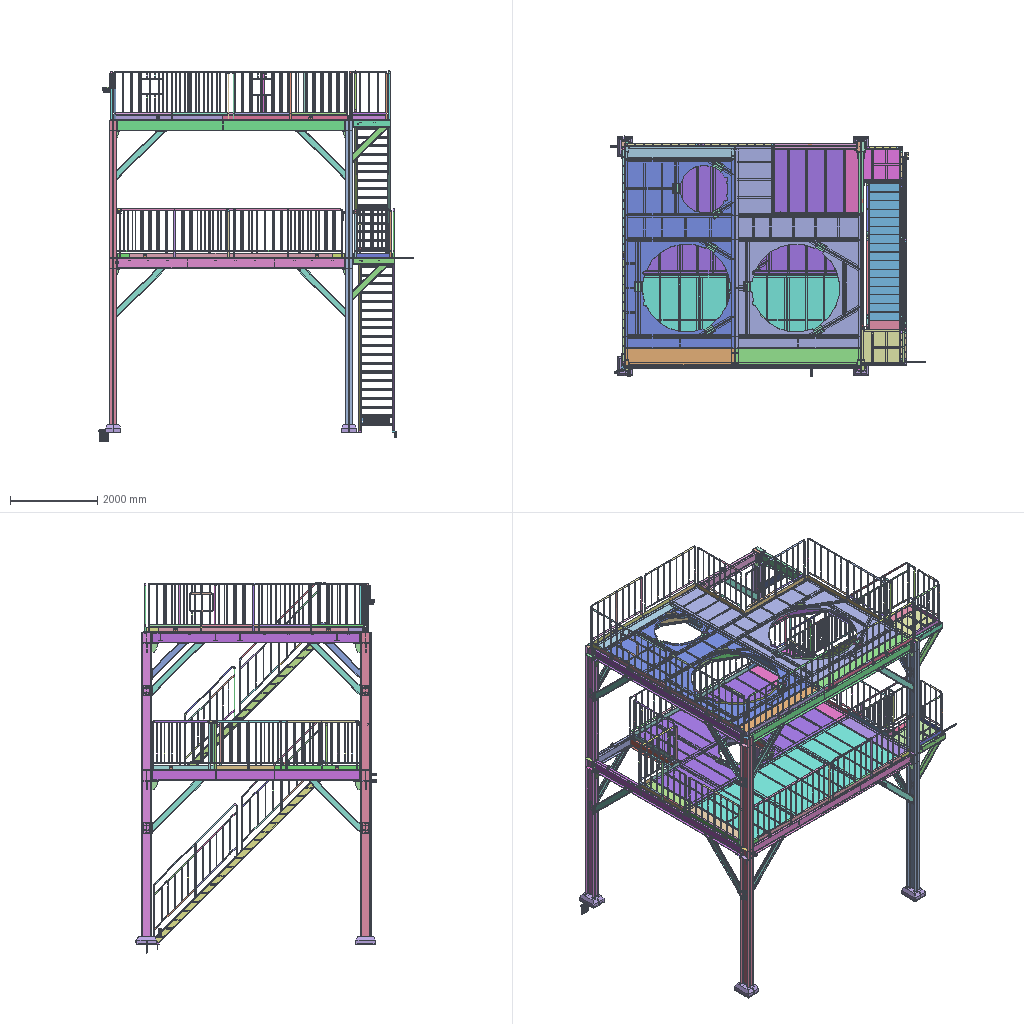Assembly | STEP file | 100 different items | 3011 placed | box 7212 x 5519 x 8479 mm
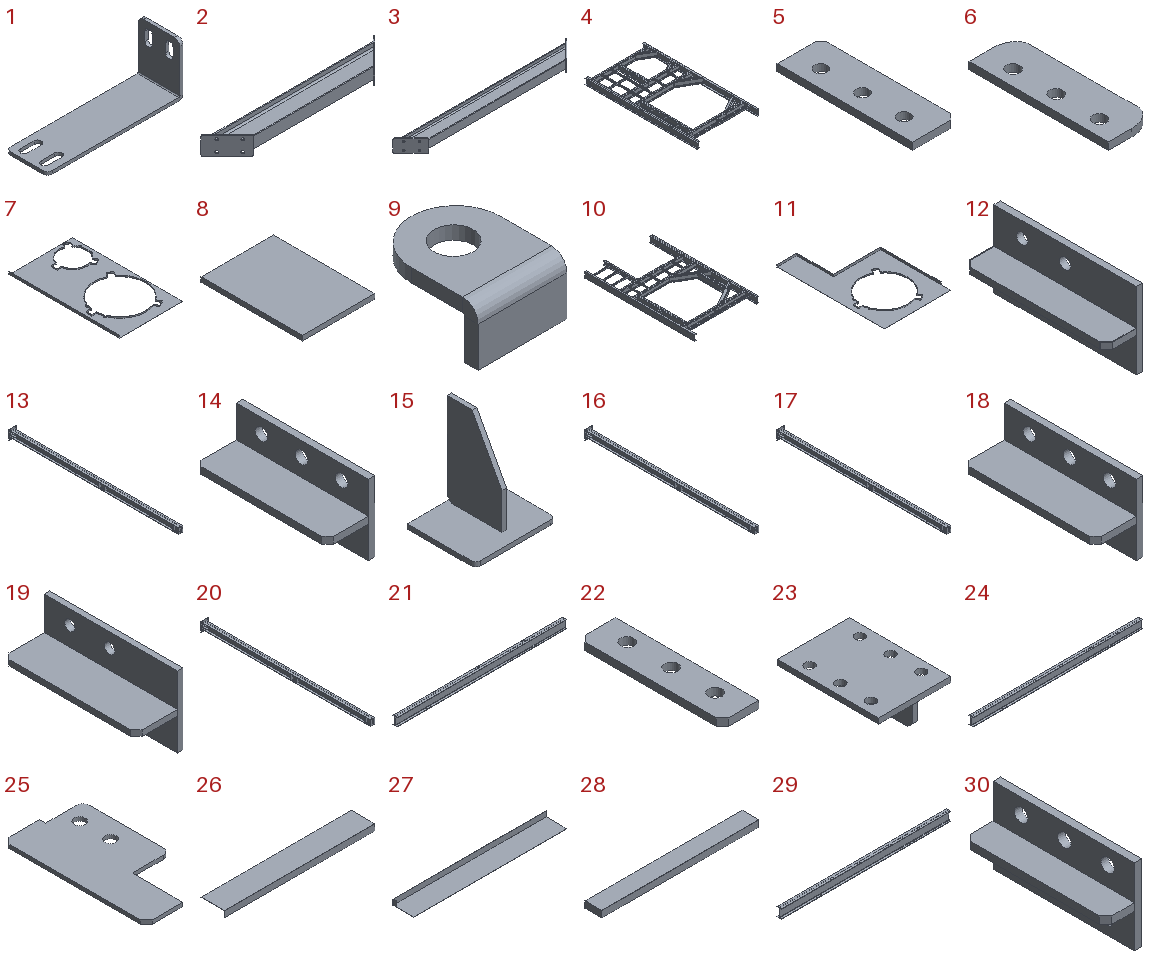Parts list (item | name | quantity | parent item | size | volume):
1 | PN_0061 L-type guardrail connecting plate 130X50_Default<As Machined> | x3 | - | 130 x 40 x 50 mm | 19703 mm3
2 | PN_0060 steel beam brace 1140_Default<As Machined> | x2 | - | 1178 x 182.434 x 125 mm | 2280023 mm3
3 | PN_0059 steel column and steel beam brace 1677_Default<As Machined> | x14 | - | 1715 x 182.434 x 125 mm | 3255129 mm3
4 | PN_0020 third-floor right platform 1_Default<As Machined> | x1 | in PN_0083 third-floor platform assembly 1 | 2578 x 4889 x 250 mm | 86538264 mm3
5 | PN_0021 flange connecting plate 12t_Default<As Machined> | x16 | in PN_0083 third-floor platform assembly 1, PN_0084 third-floor platform assembly 2, PN_0091 second-floor beam assembly, PN_0092 second-floor beam assembly 2 | 75 x 232 x 12 mm | 194530 mm3
6 | PN_0022 channel connecting plate 12t_Default<As Machined> | x8 | in PN_0083 third-floor platform assembly 1, PN_0084 third-floor platform assembly 2, PN_0093 second-floor platform assembly 1, PN_0094 second-floor platform assembly 2 | 73 x 226 x 12 mm | 180413 mm3
7 | PN_0023 third-floor right platform deck checkered steel plate_Default<As Machined> | x1 | in PN_0083 third-floor platform assembly 1 | 2515 x 4350 x 103 mm | 22833161 mm3
8 | PN_0009 support base plate 150x210_Default<As Machined> | x12 | in PN_0083 third-floor platform assembly 1, PN_0084 third-floor platform assembly 2, PN_0094 second-floor platform assembly 2 | 150 x 210 x 10 mm | 315000 mm3
9 | PN_0019 lifting lug _Default<As Machined> | x24 | in PN_0083 third-floor platform assembly 1, PN_0084 third-floor platform assembly 2, PN_0089 third-floor beam assembly 1, PN_0090 third-floor beam assembly 2, PN_0091 second-floor beam assembly, PN_0092 second-floor beam assembly 2, PN_0093 second-floor platform assembly 1, PN_0094 second-floor platform assembly 2 | 80 x 100 x 50 mm | 109398 mm3
10 | PN_0025 third-floor left platform 1_Default<As Machined> | x1 | in PN_0084 third-floor platform assembly 2 | 2948 x 4889 x 250 mm | 85593923 mm3
11 | PN_0024 third-floor left platform deck_Default<As Machined> | x1 | in PN_0084 third-floor platform assembly 2 | 2885 x 4620 x 103 mm | 23616795 mm3
12 | PN_0026 stair beam corbel 10t_Default<As Machined> | x3 | in PN_0084 third-floor platform assembly 2, PN_0092 second-floor beam assembly 2 | 59.5 x 233 x 125 mm | 507501 mm3
13 | PN_0027 steel column HM250X175=7134_Default<As Machined> | x1 | in PN_0085 column assembly 1 | 300 x 7150 x 400 mm | 42980324 mm3
14 | PN_0028 web-top 12t steel corbel_Default<As Machined> | x7 | in PN_0085 column assembly 1, PN_0086 column assembly 2, PN_0087 column assembly 3, PN_0088 column assembly 4 | 84 x 234 x 125 mm | 525836 mm3
15 | PN_0029 web-top 10t steel corbel_Default<As Machined> | x16 | in PN_0085 column assembly 1, PN_0086 column assembly 2, PN_0087 column assembly 3, PN_0088 column assembly 4 | 175 x 150 x 209.905 mm | 462571 mm3
16 | PN_0027 steel column HM250X175=7134_Default<As Machined> | x1 | in PN_0086 column assembly 2 | 300 x 7150 x 400 mm | 42979753 mm3
17 | PN_0027 steel column HM250X175=7134_Default<As Machined> | x1 | in PN_0087 column assembly 3 | 300 x 7150 x 400 mm | 42973088 mm3
18 | PN_0028 web-top 12t steel corbel_Default<As Machined> | x1 | in PN_0087 column assembly 3 | 84 x 234 x 125 mm | 525821 mm3
19 | PN_0030 stair beam corbel 10t_Default<As Machined> | x3 | in PN_0087 column assembly 3 | 82 x 234 x 125 mm | 449801 mm3
20 | PN_0027 steel column HM250X175=7134_Default<As Machined> | x1 | in PN_0088 column assembly 4 | 300 x 7150 x 400 mm | 42977522 mm3
21 | PN_0031 main beam HN250X125=5225_Default<As Machined> | x1 | in PN_0089 third-floor beam assembly 1 | 5225 x 125 x 250 mm | 19289440 mm3
22 | PN_0032 connecting plate 12t_Default<As Machined> | x20 | in PN_0089 third-floor beam assembly 1, PN_0090 third-floor beam assembly 2, PN_0093 second-floor platform assembly 1, PN_0094 second-floor platform assembly 2 | 59.5 x 232 x 12 mm | 151378 mm3
23 | PN_0033 beam connector 12t_Default<As Machined> | x4 | in PN_0089 third-floor beam assembly 1, PN_0090 third-floor beam assembly 2, PN_0091 second-floor beam assembly, PN_0092 second-floor beam assembly 2 | 164.5 x 232 x 59.5 mm | 562868 mm3
24 | PN_0031 main beam HN250X125=5225_Default<As Machined> | x1 | in PN_0090 third-floor beam assembly 2 | 5225 x 125 x 250 mm | 19288459 mm3
25 | PN_0034 channel connecting plate_Default<As Machined> | x1 | in PN_0090 third-floor beam assembly 2 | 119.5 x 232 x 6 mm | 129313 mm3
26 | PN_0035 third-floor site mounting plate 1_Default<As Machined> | x1 | - | 2515 x 394 x 103 mm | 3844530 mm3
27 | PN_0036 third-floor site mounting plate 2_Default<As Machined> | x1 | - | 2885 x 394 x 103 mm | 4292084 mm3
28 | PN_0037 third-floor site mounting plate 3_Default<As Machined> | x1 | - | 2515 x 270 x 103 mm | 2871750 mm3
29 | PN_0038 main beam HN250X125=5225_Default<As Machined> | x1 | in PN_0091 second-floor beam assembly | 4770 x 125 x 250 mm | 17605699 mm3
30 | PN_0039 web-top 12t steel corbel_Default<As Machined> | x2 | in PN_0091 second-floor beam assembly, PN_0092 second-floor beam assembly 2 | 59.5 x 232 x 125 mm | 452900 mm3
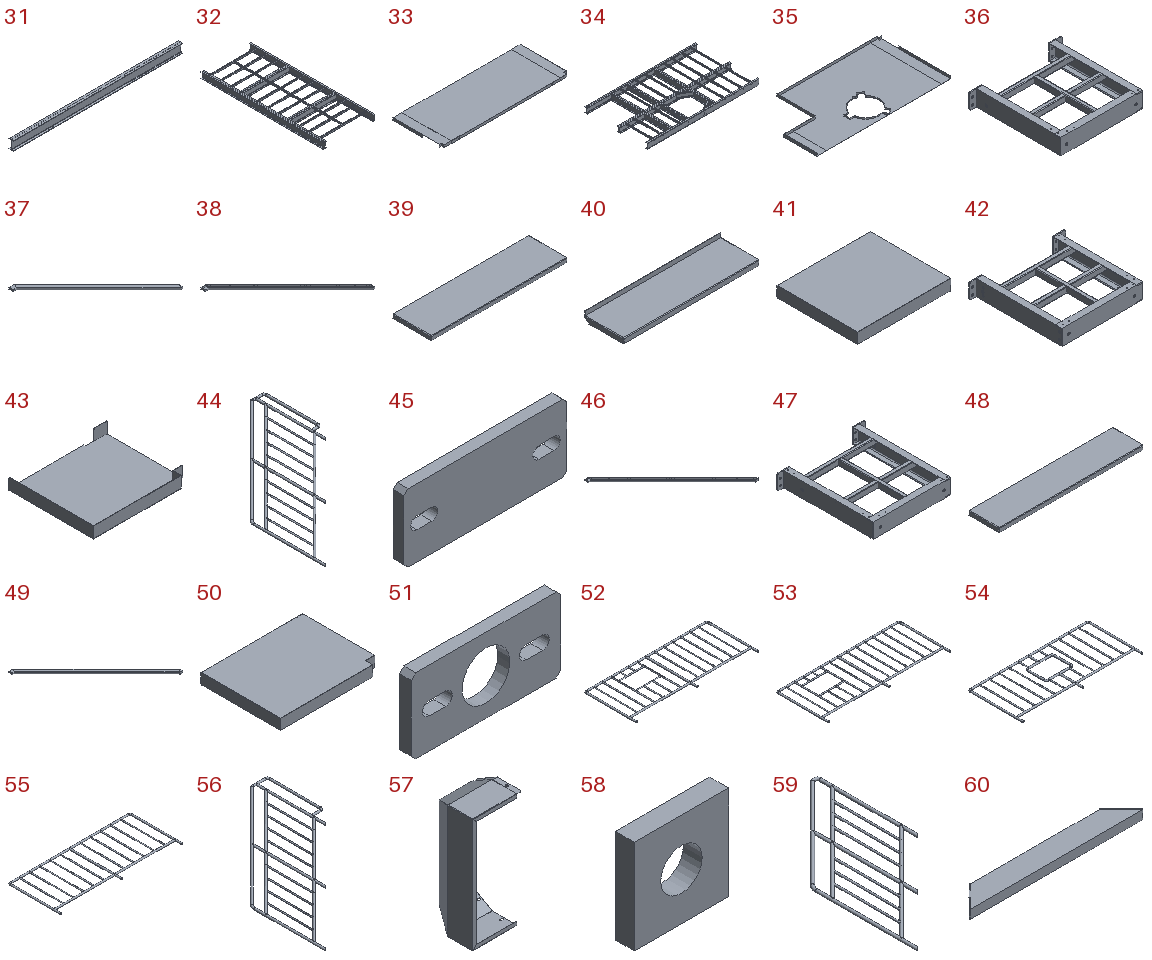31 | PN_0038 main beam HN250X125=5225_Default<As Machined> | x1 | in PN_0092 second-floor beam assembly 2 | 4770 x 125 x 250 mm | 17606026 mm3
32 | PN_0040 second-floor platform deck_Default<As Machined> | x1 | in PN_0093 second-floor platform assembly 1 | 2148 x 5275 x 250 mm | 68076276 mm3
33 | PN_0041 second-floor passage platform plate_Default<As Machined> | x1 | in PN_0093 second-floor platform assembly 1 | 5405 x 2088 x 103 mm | 36419067 mm3
34 | PN_0042 second-floor transition bin platform deck_Default<As Machined> | x1 | in PN_0094 second-floor platform assembly 2 | 5275 x 2990 x 250 mm | 103147929 mm3
35 | PN_0043 checkered steel plate 4785x1464_Default<As Machined> | x1 | in PN_0094 second-floor platform assembly 2 | 5405 x 2881 x 103 mm | 41382976 mm3
36 | PN_0044 steel stair platform_Default<As Machined> | x1 | in PN_0095 second-floor stair assembly | 951 x 886.002 x 160 mm | 6916698 mm3
37 | PN_0045 second-floor stair beam [16a_Default<As Machined> | x1 | in PN_0095 second-floor stair assembly | 3362 x 3310 x 63 mm | 10264966 mm3
38 | PN_0046 mirrored second-floor stair beam [16a_Default<As Machined> | x1 | in PN_0095 second-floor stair assembly | 3362 x 3310 x 63 mm | 10264966 mm3
39 | PN_0008 top 304 stair tread_Default<As Machined> | x1 | in PN_0095 second-floor stair assembly | 700 x 200 x 20 mm | 506035 mm3
40 | PN_0017 304 stair tread_Default<As Machined> | x35 | in PN_0095 second-floor stair assembly, PN_0098 first-floor steel stair assembly | 700 x 200 x 47 mm | 531503 mm3
41 | PN_0047 checkered steel plate 3_Default<As Machined> | x1 | in PN_0095 second-floor stair assembly | 891 x 771 x 103 mm | 2594390 mm3
42 | PN_0048 stair platform 2_Default<As Machined> | x1 | in PN_0096 stair platform assembly 2 | 951 x 886 x 160 mm | 6916619 mm3
43 | PN_0049 checkered steel plate 1_Default<As Machined> | x1 | in PN_0096 stair platform assembly 2 | 891 x 786 x 103 mm | 2627240 mm3
44 | PN_0050 stair guardrail B_Default<As Machined> | x2 | in PN_0097 first-floor stair guardrail A | 1972 x 2980 x 32 mm | 2990354 mm3
45 | PN_0013 304 stair handrail mounting plate 120X50X8_Default<As Machined> | x24 | in PN_0097 first-floor stair guardrail A, PN_0080 first-floor stair guardrail A, PN_0082 second-floor stair guardrail B, PN_0081 stair guardrail A section | 120 x 8 x 50 mm | 45254 mm3
46 | PN_0051 first-floor stair beam_Default<As Machined> | x1 | in PN_0098 first-floor steel stair assembly | 4058 x 4000 x 90 mm | 12422698 mm3
47 | PN_0052 steel stair platform 2_Default<As Machined> | x1 | in PN_0098 first-floor steel stair assembly | 951 x 986.002 x 160 mm | 7405397 mm3
48 | PN_0053 top 304 stair tread 2_Default<As Machined> | x1 | in PN_0098 first-floor steel stair assembly | 700 x 150 x 20 mm | 396167 mm3
49 | PN_0062 mirrored first-floor stair beam_Default<As Machined> | x1 | in PN_0098 first-floor steel stair assembly | 4058 x 4000 x 90 mm | 12422698 mm3
50 | PN_0054 checkered steel plate 2_Default<As Machined> | x1 | in PN_0098 first-floor steel stair assembly | 991 x 771 x 103 mm | 2887790 mm3
51 | PN_0067 304 guardrail mounting plate 100X50X8_Default<As Machined> | x67 | in PN_0099 304 guardrail 2600x1100B assembly, PN_0100 guardrail 2600x1100A assembly, PN_0101 304 guardrail 2400X1100A assembly, PN_0102 304 guardrail 2560X1100, PN_0065 304 guardrail 700X1100, PN_0079 platform deck guardrail 650x1100, PN_0076 304 guardrail 800X1100, PN_0064 304 guardrail 1950X1100, PN_0063 304 guardrail 1300X1100, PN_0070 304 guardrail 1150X1100, PN_0066 304 guardrail 1395X1100, PN_0068 304 guardrail 1880X1100, PN_0069 304 guardrail 1500X1100, PN_0078 304 guardrail 1620X1100, PN_0077 304 guardrail 2480X1100, PN_0075 304 guardrail 2400X1100 | 100 x 8 x 50 mm | 30820 mm3
52 | PN_0055 304 guardrail 2600X1100_Default<As Machined> | x1 | in PN_0099 304 guardrail 2600x1100B assembly | 2632 x 1116 x 32 mm | 2872572 mm3
53 | PN_0056 304 guardrail 2600X1100B_Default<As Machined> | x1 | in PN_0100 guardrail 2600x1100A assembly | 2632 x 1116 x 32 mm | 2870828 mm3
54 | PN_0057 304 guardrail 2400X1100 body A_Default<As Machined> | x1 | in PN_0101 304 guardrail 2400X1100A assembly | 2432 x 1116 x 32 mm | 2712212 mm3
55 | PN_0058 304 guardrail 2560X1100 body-A_Default<As Machined> | x1 | in PN_0102 304 guardrail 2560X1100 | 2592 x 1116 x 32 mm | 2611653 mm3
56 | PN_0012 stair guardrail B_Default<As Machined> | x2 | in PN_0080 first-floor stair guardrail A | 2022 x 2980 x 32 mm | 3009194 mm3
57 | PN_0018 H244x175 column protective cover_Default<As Machined> | x8 | - | 195 x 178.808 x 450 mm | 198447 mm3
58 | PN_0016 anchor bolt shim_Default<As Machined> | x40 | - | 50 x 10 x 50 mm | 21199 mm3
59 | PN_0015 second-floor stair guardrail A_Default<As Machined> | x2 | in PN_0082 second-floor stair guardrail B | 1170 x 2330 x 32 mm | 2093979 mm3
60 | PN_0010 stair platform brace 1257_Default<As Machined> | x3 | - | 1268 x 165.463 x 63 mm | 2607828 mm3
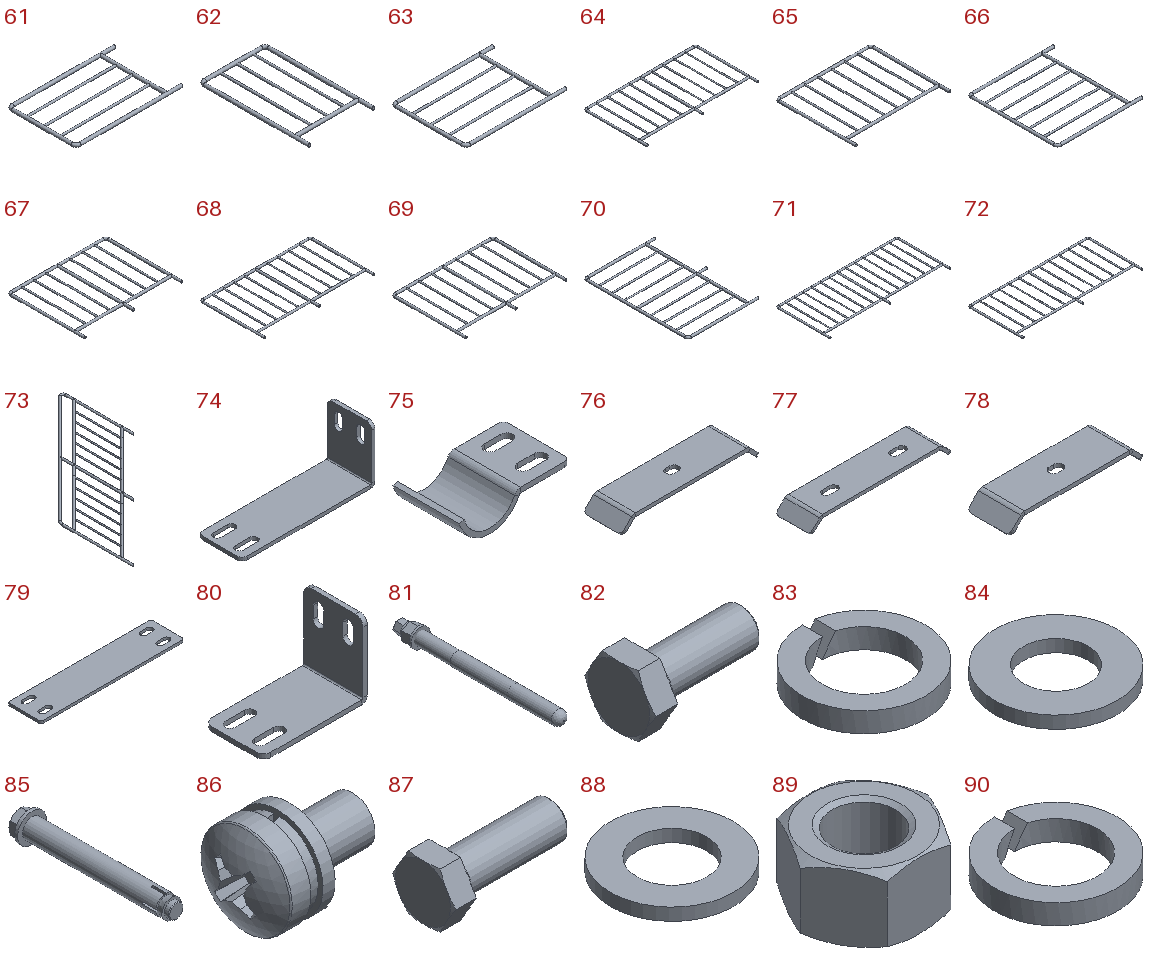61 | 304 guardrail 700X1100 body_Default<As Machined> | x1 | in PN_0065 304 guardrail 700X1100 | 1116 x 732 x 32 mm | 674327 mm3
62 | PN_0011 platform deck 304 guardrail 650X1100_Default<As Machined> | x3 | in PN_0079 platform deck guardrail 650x1100 | 682 x 1116 x 32 mm | 971799 mm3
63 | PN_0003 304 guardrail 800X1100 body-A_Default<As Machined> | x2 | in PN_0076 304 guardrail 800X1100 | 1116 x 832 x 32 mm | 1018076 mm3
64 | 304 guardrail 1950X1100-D body_Default<As Machined> | x2 | in PN_0064 304 guardrail 1950X1100 | 1982 x 1116 x 32 mm | 1461752 mm3
65 | 304 guardrail 1300X1100 body-B_Default<As Machined> | x1 | in PN_0063 304 guardrail 1300X1100 | 1332 x 1116 x 32 mm | 1011632 mm3
66 | 304 guardrail 1150X1100 body_Default<As Machined> | x1 | in PN_0070 304 guardrail 1150X1100 | 1116 x 1182 x 32 mm | 913541 mm3
67 | 304 guardrail 1395X1100 body B_Default<As Machined> | x1 | in PN_0066 304 guardrail 1395X1100 | 1427 x 1116 x 32 mm | 1755808 mm3
68 | 304 guardrail 1880X1100 body_Default<As Machined> | x1 | in PN_0068 304 guardrail 1880X1100 | 1912 x 1116 x 32 mm | 1441532 mm3
69 | 304 guardrail 1500X1100-B_Default<As Machined> | x2 | in PN_0069 304 guardrail 1500X1100 | 1532 x 1116 x 32 mm | 1222525 mm3
70 | PN_0005 guardrail 1620X1100 body_Default<As Machined> | x4 | in PN_0078 304 guardrail 1620X1100 | 1116 x 1652 x 32 mm | 1256893 mm3
71 | PN_0004 304 guardrail 2480X1100 body_Default<As Machined> | x2 | in PN_0077 304 guardrail 2480X1100 | 2512 x 1116 x 32 mm | 1834535 mm3
72 | PN_0002 304 guardrail 2400X1100 body-B_Default<As Machined> | x1 | in PN_0075 304 guardrail 2400X1100 | 2432 x 1116 x 32 mm | 2551384 mm3
73 | PN_0014 stair guardrail A_Default<As Machined> | x2 | in PN_0081 stair guardrail A section | 1927 x 3087 x 32 mm | 3023959 mm3
74 | PN_0007 L-type guardrail connecting plate 120X50_Default<As Machined> | x2 | - | 120 x 40 x 50 mm | 18503 mm3
75 | PN_0001 guardrail connecting plate 1_Default<As Machined> | x16 | in PN_0108 guardrail connection assembly 32 | 66.397 x 40 x 15 mm | 8448 mm3
76 | PN_0074 guardrail connecting plate (spacing 120)_Default<As Machined> | x120 | in PN_0110 guardrail connection assembly (spacing 120) 201 | 164.912 x 45 x 17 mm | 30539 mm3
77 | PN_0071 guardrail connecting plate (spacing 140)_Default<As Machined> | x12 | in PN_0107 guardrail connection assembly (spacing 140) 201 | 184.912 x 45 x 17 mm | 33225 mm3
78 | PN_0073 guardrail connecting plate (spacing 100)_Default<As Machined> | x16 | in PN_0109 guardrail connection assembly (spacing 100) 201 | 144.912 x 45 x 17 mm | 26939 mm3
79 | PN_0006 guardrail connecting plate 210_Default<As Machined> | x1 | - | 170 x 40 x 3 mm | 19243 mm3
80 | PN_0072 L-type guardrail connecting plate 70X50_Default<As Machined> | x1 | - | 70 x 40 x 50 mm | 12503 mm3
81 | Chemical anchor bolt M20X260 8.8 JBZQ4757-2006_Default<As Machined> | x40 | - | 30 x 262 x 30 mm | 79535 mm3
82 | Hex head bolt M8X20 A2-70 GBT5783-2016_GB_FASTENER_BOLT_STBAB A M8X20-N | x180 | in PN_0105 hex head bolt set M8X20 | 25.45 x 14.699 x 12.73 mm | 1753 mm3
83 | Spring washer 8 A2-70 GBT93-1987_GB_FASTENER_WASHER_SW 8 | x180 | in PN_0105 hex head bolt set M8X20 | 12.88 x 12.88 x 2.1 mm | 143.98 mm3
84 | Flat washer 8 A2-70 GBT97.1-2002_GB_FASTENER_WASHER_PWNA 8 | x240 | in PN_0105 hex head bolt set M8X20, PN_0106 hex head bolt set M8X50 | 16 x 16 x 1.6 mm | 233.031 mm3
85 | Cone-head expansion bolt (ZM type) M12×110 A2-70 GBT22795 (ZM) - 2008_Default<As Machined> | x6 | - | 24 x 129.18 x 24 mm | 26435 mm3
86 | Cross recessed pan head combination screw M6×12 A2-70 GBT9074.4-1988 | x20 | - | 16.483 x 12 x 12 mm | 913.256 mm3
87 | Hex head bolt M16X45 A2-70 GBT5783-2016_GB_FASTENER_BOLT_STBAB A M16X45-N | x200 | - | 55.18 x 27.332 x 23.67 mm | 13915 mm3
88 | Flat washer 16 A2-70 GBT97.1-2002_GB_FASTENER_WASHER_PWNA 16 | x200 | - | 30 x 30 x 3 mm | 1440 mm3
89 | Hex nut M16 A2-70 GBT6170-2015_GB_FASTENER_NUT_SNAB1 M16-N | x200 | - | 27.713 x 24 x 14.8 mm | 5071 mm3
90 | Spring washer 16 A2-70 GBT93-1987_GB_FASTENER_WASHER_SW 16 | x200 | - | 25.1 x 25.1 x 4.1 mm | 1069 mm3
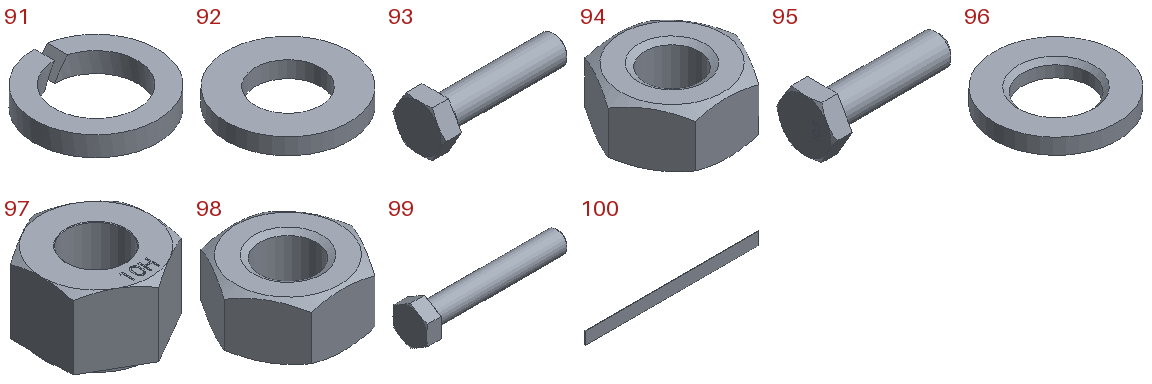91 | Spring washer 6 A2-70 GBT93-1987_GB_FASTENER_WASHER_SW 6 | x40 | in PN_0103 hex head bolt set M6X25 | 9.88 x 9.88 x 1.6 mm | 64.217 mm3
92 | Flat washer 6 A2-70 GBT97.1-2002_GB_FASTENER_WASHER_PWNA 6 | x40 | in PN_0103 hex head bolt set M6X25 | 12 x 12 x 1.6 mm | 129.484 mm3
93 | Hex head bolt M6X25 A2-70 GBT5783-2016_GB_FASTENER_BOLT_STBAB A M6X25-N | x40 | in PN_0103 hex head bolt set M6X25 | 29.15 x 11.293 x 9.78 mm | 1042 mm3
94 | Hex nut M6 A2-70 GBT6170-2015_GB_FASTENER_NUT_SNAB1 M6-N | x40 | in PN_0103 hex head bolt set M6X25 | 11.547 x 10 x 5.2 mm | 340.667 mm3
95 | Hex head bolt for steel structures M16×60 10.9 GBT1228-2006_M16×55 | x160 | in PN_0104 large hex head bolt set for steel structures M16X60 | 70.1 x 31.177 x 27 mm | 18177 mm3
96 | Washer for steel structures 16 GBT1230-2006_16 | x320 | in PN_0104 large hex head bolt set for steel structures M16X60 | 31.4 x 31.4 x 4 mm | 2155 mm3
97 | Hex nut for steel structures M16 10H GBT1229-2006_M16 | x160 | in PN_0104 large hex head bolt set for steel structures M16X60 | 25.6 x 29.56 x 17.2 mm | 7051 mm3
98 | Hex nut M8 A2-70 GBT6170-2015_GB_FASTENER_NUT_SNAB1 M8-N | x60 | in PN_0106 hex head bolt set M8X50 | 15.011 x 13 x 6.8 mm | 739.531 mm3
99 | Hex head bolt M8X50 A2-70 GBT5782-2016_GB_FASTENER_BOLT_SB A M8X40-C | x60 | in PN_0106 hex head bolt set M8X50 | 55.95 x 12.73 x 14.699 mm | 3330 mm3
100 | Stair anti-slip strip_Default<As Machined> | x80 | - | 700 x 3 x 50 mm | 105000 mm3
Placements (level | parent | child | x y z in mm | rotation matrix by rows), first 168 of 3581 lines:
1 | subassembly 2 | PN_0061 L-type guardrail connecting plate 130X50_Default<As Machined> | 4634.399 -2825.874 2881.2 | 1 0 0 0 0 -1 0 1 0
1 | subassembly 2 | PN_0061 L-type guardrail connecting plate 130X50_Default<As Machined> | 4634.399 2213.126 2881.2 | 1 0 0 0 0 -1 0 1 0
1 | subassembly 2 | PN_0061 L-type guardrail connecting plate 130X50_Default<As Machined> | -628.601 -2820.874 2881.2 | -1 0 0 0 0 -1 0 -1 -0
1 | subassembly 2 | PN_0060 steel beam brace 1140_Default<As Machined> | 4702.899 1802.641 4434.215 | 0 0 -1 0.7071 -0.7071 0 -0.7071 -0.7071 -0
1 | subassembly 2 | PN_0060 steel beam brace 1140_Default<As Machined> | 4702.899 -2357.389 4434.215 | 0 0 1 -0.7071 0.7071 0 -0.7071 -0.7071 -0
1 | subassembly 2 | PN_0059 steel column and steel beam brace 1677_Default<As Machined> | 4702.899 1612.783 1094.357 | 0 0 -1 0.7071 -0.7071 0 -0.7071 -0.7071 -0
1 | subassembly 2 | PN_0059 steel column and steel beam brace 1677_Default<As Machined> | 4702.899 -2167.531 1094.357 | 0 0 1 -0.7071 0.7071 0 -0.7071 -0.7071 0
1 | subassembly 2 | PN_0059 steel column and steel beam brace 1677_Default<As Machined> | 4204.556 -2784.374 1094.357 | 0.7071 -0.7071 0 0 0 1 -0.7071 -0.7071 -0
1 | subassembly 2 | PN_0059 steel column and steel beam brace 1677_Default<As Machined> | -697.101 -2167.531 1094.357 | 0 0 1 -0.7071 0.7071 0 -0.7071 -0.7071 -0
1 | subassembly 2 | PN_0059 steel column and steel beam brace 1677_Default<As Machined> | -198.758 2229.626 1094.357 | -0.7071 0.7071 0 0 0 -1 -0.7071 -0.7071 0
1 | subassembly 2 | PN_0059 steel column and steel beam brace 1677_Default<As Machined> | 4204.556 2229.626 1094.357 | 0.7071 -0.7071 0 0 0 1 -0.7071 -0.7071 -0
1 | subassembly 2 | PN_0059 steel column and steel beam brace 1677_Default<As Machined> | -198.758 -2784.374 1094.357 | -0.7071 0.7071 0 0 0 -1 -0.7071 -0.7071 0
1 | subassembly 2 | PN_0059 steel column and steel beam brace 1677_Default<As Machined> | -697.101 1612.783 1094.357 | 0 0 -1 0.7071 -0.7071 0 -0.7071 -0.7071 -0
1 | subassembly 2 | PN_0083 third-floor platform assembly 1 | 1225.628 -145.413 44.2 | 1 0 0 0 1 0 0 0 1
2 | PN_0083 third-floor platform assembly 1 | PN_0020 third-floor right platform 1_Default<As Machined> | -517.729 -869.961 4695.0 | 1 0 0 0 1 0 0 0 1
2 | PN_0083 third-floor platform assembly 1 | PN_0021 flange connecting plate 12t_Default<As Machined> | -1963.229 -2504.961 4820.0 | 1 0 0 0 0 -1 0 1 -0
2 | PN_0083 third-floor platform assembly 1 | PN_0021 flange connecting plate 12t_Default<As Machined> | -1882.229 -2516.961 4820.0 | -1 0 0 0 0 1 0 1 0
2 | PN_0083 third-floor platform assembly 1 | PN_0021 flange connecting plate 12t_Default<As Machined> | -1882.229 2253.039 4820.0 | -1 0 0 0 0 -1 0 -1 -0
2 | PN_0083 third-floor platform assembly 1 | PN_0021 flange connecting plate 12t_Default<As Machined> | -1963.229 2241.039 4820.0 | 1 0 0 0 0 1 0 -1 -0
2 | PN_0083 third-floor platform assembly 1 | PN_0022 channel connecting plate 12t_Default<As Machined> | 546.771 -2564.461 4820.0 | 1 0 0 0 0 -1 0 1 -0
2 | PN_0083 third-floor platform assembly 1 | PN_0022 channel connecting plate 12t_Default<As Machined> | 546.771 2312.539 4820.0 | 1 0 0 0 0 -1 0 1 -0
2 | PN_0083 third-floor platform assembly 1 | PN_0023 third-floor right platform deck checkered steel plate_Default<As Machined> | -517.729 -869.961 4948.0 | 1 0 0 0 1 0 0 0 1
2 | PN_0083 third-floor platform assembly 1 | PN_0009 support base plate 150x210_Default<As Machined> | 7.54 -1839.754 4955.0 | 0.5 -0.866 0 -0.866 -0.5 0 0 0 -1
2 | PN_0083 third-floor platform assembly 1 | PN_0009 support base plate 150x210_Default<As Machined> | -741.614 1419.392 4955.0 | 1 0 0 0 -1 0 0 0 -1
2 | PN_0083 third-floor platform assembly 1 | PN_0009 support base plate 150x210_Default<As Machined> | 59.502 69.832 4955.0 | 0.5 0.866 0 0.866 -0.5 0 0 0 -1
2 | PN_0083 third-floor platform assembly 1 | PN_0009 support base plate 150x210_Default<As Machined> | -1620.229 -839.961 4955.0 | -1 0 0 0 1 0 0 0 -1
2 | PN_0083 third-floor platform assembly 1 | PN_0009 support base plate 150x210_Default<As Machined> | 173.124 842.562 4955.0 | -0.5 0.866 0 0.866 0.5 0 0 0 -1
2 | PN_0083 third-floor platform assembly 1 | PN_0009 support base plate 150x210_Default<As Machined> | 215.304 1923.164 4955.0 | -0.5 -0.866 0 -0.866 0.5 0 0 0 -1
2 | PN_0083 third-floor platform assembly 1 | PN_0019 lifting lug _Default<As Machined> | -1947.729 1713.039 4957.0 | 0 0 1 1 0 0 0 1 0
2 | PN_0083 third-floor platform assembly 1 | PN_0019 lifting lug _Default<As Machined> | 571.271 2167.539 4880.118 | 0 -1 0 0 0 -1 1 0 0
2 | PN_0083 third-floor platform assembly 1 | PN_0019 lifting lug _Default<As Machined> | -1947.729 -1786.961 4957.0 | 0 0 1 1 0 0 0 1 0
2 | PN_0083 third-floor platform assembly 1 | PN_0019 lifting lug _Default<As Machined> | 571.271 -2332.461 4880.118 | 0 -1 0 0 0 -1 1 0 0
1 | subassembly 2 | PN_0084 third-floor platform assembly 2 | 3923.757 -499.454 44.2 | 1 0 0 0 1 0 0 0 1
2 | PN_0084 third-floor platform assembly 2 | PN_0025 third-floor left platform 1_Default<As Machined> | -715.858 -515.92 4695.0 | 1 0 0 0 1 0 0 0 1
2 | PN_0084 third-floor platform assembly 2 | PN_0021 flange connecting plate 12t_Default<As Machined> | 738.642 -2150.92 4820.0 | 1 0 0 0 0 -1 0 1 0
2 | PN_0084 third-floor platform assembly 2 | PN_0021 flange connecting plate 12t_Default<As Machined> | 819.642 -2150.92 4820.0 | -1 0 0 0 0 -1 0 -1 0
2 | PN_0084 third-floor platform assembly 2 | PN_0021 flange connecting plate 12t_Default<As Machined> | 819.642 2595.08 4820.0 | -1 0 0 0 0 1 0 1 0
2 | PN_0084 third-floor platform assembly 2 | PN_0021 flange connecting plate 12t_Default<As Machined> | 738.642 2607.08 4820.0 | 1 0 0 0 0 -1 0 1 -0
2 | PN_0084 third-floor platform assembly 2 | PN_0022 channel connecting plate 12t_Default<As Machined> | -2060.358 2654.58 4820.0 | -1 0 0 0 0 1 0 1 -0
2 | PN_0084 third-floor platform assembly 2 | PN_0022 channel connecting plate 12t_Default<As Machined> | -2060.358 -2222.42 4820.0 | -1 0 0 0 0 1 0 1 -0
2 | PN_0084 third-floor platform assembly 2 | PN_0024 third-floor left platform deck_Default<As Machined> | -715.858 -515.92 4948.0 | 1 0 0 0 1 0 0 0 1
2 | PN_0084 third-floor platform assembly 2 | PN_0009 support base plate 150x210_Default<As Machined> | -190.589 -1485.713 4945.0 | 0.5 0.866 0 -0.866 0.5 0 0 0 1
2 | PN_0084 third-floor platform assembly 2 | PN_0009 support base plate 150x210_Default<As Machined> | -138.627 423.873 4945.0 | 0.5 -0.866 0 0.866 0.5 0 0 0 1
2 | PN_0084 third-floor platform assembly 2 | PN_0009 support base plate 150x210_Default<As Machined> | -1818.358 -485.92 4945.0 | -1 0 0 0 -1 0 0 0 1
2 | PN_0084 third-floor platform assembly 2 | PN_0019 lifting lug _Default<As Machined> | 804.142 -1222.92 4957.0 | 0 0 -1 -1 0 0 0 1 0
2 | PN_0084 third-floor platform assembly 2 | PN_0019 lifting lug _Default<As Machined> | -2084.858 -2027.42 4880.118 | 0 1 0 0 0 1 1 0 -0
2 | PN_0084 third-floor platform assembly 2 | PN_0019 lifting lug _Default<As Machined> | -1080.858 1158.83 4884.0 | 0 0 1 0 1 0 -1 0 0
2 | PN_0084 third-floor platform assembly 2 | PN_0019 lifting lug _Default<As Machined> | 804.142 1477.08 4957.0 | 0 0 -1 -1 0 0 0 1 0
2 | PN_0084 third-floor platform assembly 2 | PN_0026 stair beam corbel 10t_Default<As Machined> | 806.892 -1452.971 4819 | 1 0 0 0 0 -1 0 1 0
1 | subassembly 2 | PN_0085 column assembly 1 | -697.101 2229.626 4989.2 | 1 0 0 0 0 1 0 -1 -0
2 | PN_0085 column assembly 1 | PN_0027 steel column HM250X175=7134_Default<As Machined> | -0.0 -0.0 -0.0 | 1 0 0 0 1 0 0 0 1
2 | PN_0085 column assembly 1 | PN_0028 web-top 12t steel corbel_Default<As Machined> | 39.5 125 6.004 | 1 0 0 0 -1 0 0 0 -1
2 | PN_0085 column assembly 1 | PN_0029 web-top 10t steel corbel_Default<As Machined> | 78.5 250.0 0.0 | 0 -1 0 0 0 1 -1 0 0
2 | PN_0085 column assembly 1 | PN_0028 web-top 12t steel corbel_Default<As Machined> | 39.5 3275 6.004 | 1 0 0 0 -1 0 0 0 -1
2 | PN_0085 column assembly 1 | PN_0029 web-top 10t steel corbel_Default<As Machined> | 78.5 3400.0 0.0 | 0 -1 0 0 0 1 -1 0 0
2 | PN_0085 column assembly 1 | PN_0029 web-top 10t steel corbel_Default<As Machined> | -0.0 250.0 -197.0 | -1 0 0 0 0 1 0 1 0
2 | PN_0085 column assembly 1 | PN_0029 web-top 10t steel corbel_Default<As Machined> | -0.0 3400.0 -197.0 | -1 0 0 0 0 1 0 1 0
1 | subassembly 2 | PN_0086 column assembly 2 | -950.144 4365.626 1027.473 | -1 0 0 0 0 -1 0 -1 0
2 | PN_0086 column assembly 2 | PN_0027 steel column HM250X175=7134_Default<As Machined> | -253.044 -3961.727 7150.0 | 1 0 0 0 1 0 0 0 1
2 | PN_0086 column assembly 2 | PN_0028 web-top 12t steel corbel_Default<As Machined> | -292.544 -3836.727 7143.996 | -1 0 0 0 -1 0 0 0 1
2 | PN_0086 column assembly 2 | PN_0029 web-top 10t steel corbel_Default<As Machined> | -331.541 -3711.727 7150.0 | 0 1 0 0 0 1 1 0 -0
2 | PN_0086 column assembly 2 | PN_0028 web-top 12t steel corbel_Default<As Machined> | -292.544 -686.727 7143.996 | -1 0 0 0 -1 0 0 0 1
2 | PN_0086 column assembly 2 | PN_0029 web-top 10t steel corbel_Default<As Machined> | -331.541 -561.727 7150.0 | 0 1 0 0 0 1 1 0 -0
2 | PN_0086 column assembly 2 | PN_0029 web-top 10t steel corbel_Default<As Machined> | -253.044 -3711.727 6953.0 | -1 0 0 0 0 1 0 1 0
2 | PN_0086 column assembly 2 | PN_0029 web-top 10t steel corbel_Default<As Machined> | -253.044 -561.727 6953.0 | -1 0 0 0 0 1 0 1 0
1 | subassembly 2 | PN_0087 column assembly 3 | 4449.855 4365.626 1027.473 | -1 0 0 0 0 -1 0 -1 -0
2 | PN_0087 column assembly 3 | PN_0027 steel column HM250X175=7134_Default<As Machined> | -253.044 -3961.727 7150.0 | 1 0 0 0 1 0 0 0 1
2 | PN_0087 column assembly 3 | PN_0028 web-top 12t steel corbel_Default<As Machined> | -213.544 -3836.727 7156.004 | 1 0 0 0 -1 0 0 0 -1
2 | PN_0087 column assembly 3 | PN_0029 web-top 10t steel corbel_Default<As Machined> | -174.544 -3711.727 7150.0 | 0 -1 0 0 0 1 -1 0 0
2 | PN_0087 column assembly 3 | PN_0028 web-top 12t steel corbel_Default<As Machined> | -213.544 -686.727 7156.004 | 1 0 0 0 -1 0 0 0 -1
2 | PN_0087 column assembly 3 | PN_0029 web-top 10t steel corbel_Default<As Machined> | -174.544 -561.727 7150.0 | 0 -1 0 0 0 1 -1 0 0
2 | PN_0087 column assembly 3 | PN_0029 web-top 10t steel corbel_Default<As Machined> | -253.044 -3711.727 6953.0 | -1 0 0 0 0 1 0 1 0
2 | PN_0087 column assembly 3 | PN_0029 web-top 10t steel corbel_Default<As Machined> | -253.044 -561.727 6953.0 | -1 0 0 0 0 1 0 1 0
2 | PN_0087 column assembly 3 | PN_0030 stair beam corbel 10t_Default<As Machined> | -294.544 -3836.727 7143.996 | -1 0 0 0 -1 0 0 0 1
2 | PN_0087 column assembly 3 | PN_0030 stair beam corbel 10t_Default<As Machined> | -294.544 -686.727 7143.996 | -1 0 0 0 -1 0 0 0 1
1 | subassembly 2 | PN_0088 column assembly 4 | 4955.943 -4920.374 1027.473 | 1 0 0 0 0 1 0 -1 -0
2 | PN_0088 column assembly 4 | PN_0027 steel column HM250X175=7134_Default<As Machined> | -253.044 -3961.727 7150.0 | 1 0 0 0 1 0 0 0 1
2 | PN_0088 column assembly 4 | PN_0028 web-top 12t steel corbel_Default<As Machined> | -292.544 -3836.727 7143.996 | -1 0 0 0 -1 0 0 0 1
2 | PN_0088 column assembly 4 | PN_0029 web-top 10t steel corbel_Default<As Machined> | -331.541 -3711.727 7150.0 | 0 1 0 0 0 1 1 0 -0
2 | PN_0088 column assembly 4 | PN_0028 web-top 12t steel corbel_Default<As Machined> | -292.544 -686.727 7143.996 | -1 0 0 0 -1 0 0 0 1
2 | PN_0088 column assembly 4 | PN_0029 web-top 10t steel corbel_Default<As Machined> | -331.541 -561.727 7150.0 | 0 1 0 0 0 1 1 0 -0
2 | PN_0088 column assembly 4 | PN_0029 web-top 10t steel corbel_Default<As Machined> | -253.044 -3711.727 6953.0 | -1 0 0 0 0 1 0 1 0
2 | PN_0088 column assembly 4 | PN_0029 web-top 10t steel corbel_Default<As Machined> | -253.044 -561.727 6953.0 | -1 0 0 0 0 1 0 1 0
1 | subassembly 2 | PN_0089 third-floor beam assembly 1 | 1784.52 -2781.678 -360.8 | -1 0 0 0 -1 0 0 0 1
2 | PN_0089 third-floor beam assembly 1 | PN_0031 main beam HN250X125=5225_Default<As Machined> | -2830.879 2.696 5225.0 | 1 0 0 0 1 0 0 0 1
2 | PN_0089 third-floor beam assembly 1 | PN_0032 connecting plate 12t_Default<As Machined> | -2830.879 35.446 5225.0 | 0 0 1 1 0 0 0 1 -0
2 | PN_0089 third-floor beam assembly 1 | PN_0032 connecting plate 12t_Default<As Machined> | 2382.121 35.446 5225.0 | 0 0 1 1 0 0 0 1 0
2 | PN_0089 third-floor beam assembly 1 | PN_0032 connecting plate 12t_Default<As Machined> | 2394.121 -30.054 5225.0 | 0 0 -1 -1 0 0 0 1 0
2 | PN_0089 third-floor beam assembly 1 | PN_0032 connecting plate 12t_Default<As Machined> | -2818.879 -30.054 5225.0 | 0 0 -1 -1 0 0 0 1 0
2 | PN_0089 third-floor beam assembly 1 | PN_0033 beam connector 12t_Default<As Machined> | -33.629 -47.804 5225.0 | 1 0 0 0 0 -1 0 1 -0
2 | PN_0089 third-floor beam assembly 1 | PN_0019 lifting lug _Default<As Machined> | -2040.879 30.196 5362.0 | 1 0 0 0 0 -1 0 1 -0
2 | PN_0089 third-floor beam assembly 1 | PN_0019 lifting lug _Default<As Machined> | 1459.121 30.196 5362.0 | 1 0 0 0 0 -1 0 1 -0
1 | subassembly 2 | PN_0090 third-floor beam assembly 2 | 1784.52 2232.322 -360.8 | -1 0 0 0 -1 0 0 0 1
2 | PN_0090 third-floor beam assembly 2 | PN_0031 main beam HN250X125=5225_Default<As Machined> | -2830.879 2.696 5225.0 | 1 0 0 0 1 0 0 0 1
2 | PN_0090 third-floor beam assembly 2 | PN_0032 connecting plate 12t_Default<As Machined> | -2830.879 35.446 5225.0 | 0 0 1 1 0 0 0 1 -0
2 | PN_0090 third-floor beam assembly 2 | PN_0032 connecting plate 12t_Default<As Machined> | 2382.121 35.446 5225.0 | 0 0 1 1 0 0 0 1 -0
2 | PN_0090 third-floor beam assembly 2 | PN_0032 connecting plate 12t_Default<As Machined> | 2394.121 -30.054 5225.0 | 0 0 -1 -1 0 0 0 1 0
2 | PN_0090 third-floor beam assembly 2 | PN_0032 connecting plate 12t_Default<As Machined> | -2818.879 -30.054 5225.0 | 0 0 -1 -1 0 0 0 1 0
2 | PN_0090 third-floor beam assembly 2 | PN_0033 beam connector 12t_Default<As Machined> | -33.629 53.196 5225.0 | -1 0 0 0 0 1 0 1 0
2 | PN_0090 third-floor beam assembly 2 | PN_0034 channel connecting plate_Default<As Machined> | -939.879 35.446 5225.0 | 0 0 1 1 0 0 0 1 -0
2 | PN_0090 third-floor beam assembly 2 | PN_0019 lifting lug _Default<As Machined> | 1754.121 -25.304 5362.0 | -1 0 0 0 0 1 0 1 0
2 | PN_0090 third-floor beam assembly 2 | PN_0019 lifting lug _Default<As Machined> | -1745.879 -25.304 5362.0 | -1 0 0 0 0 1 0 1 0
1 | subassembly 2 | PN_0035 third-floor site mounting plate 1_Default<As Machined> | 560.399 -2587.374 4989.2 | -1 0 0 0 1 0 0 0 -1
1 | subassembly 2 | PN_0036 third-floor site mounting plate 2_Default<As Machined> | 3260.399 -2587.374 4992.2 | -1 0 0 0 -1 0 0 0 1
1 | subassembly 2 | PN_0037 third-floor site mounting plate 3_Default<As Machined> | 560.399 2094.626 4989.2 | 1 0 0 0 -1 0 0 0 -1
1 | subassembly 2 | PN_0091 second-floor beam assembly | -1064.065 -2011.314 -3510.8 | 0 1 0 -1 0 0 0 0 1
2 | PN_0091 second-floor beam assembly | PN_0038 main beam HN250X125=5225_Default<As Machined> | -4118.94 366.964 5225.0 | 1 0 0 0 1 0 0 0 1
2 | PN_0091 second-floor beam assembly | PN_0021 flange connecting plate 12t_Default<As Machined> | -4106.94 407.464 5225.0 | 0 0 -1 -1 0 0 0 1 0
2 | PN_0091 second-floor beam assembly | PN_0021 flange connecting plate 12t_Default<As Machined> | -4118.94 326.464 5225.0 | 0 0 1 1 0 0 0 1 0
2 | PN_0091 second-floor beam assembly | PN_0021 flange connecting plate 12t_Default<As Machined> | 651.06 407.464 5225.0 | 0 0 -1 -1 0 0 0 1 0
2 | PN_0091 second-floor beam assembly | PN_0021 flange connecting plate 12t_Default<As Machined> | 639.06 326.464 5225.0 | 0 0 1 1 0 0 0 1 0
2 | PN_0091 second-floor beam assembly | PN_0033 beam connector 12t_Default<As Machined> | -1312.687 417.464 5225.0 | 1 0 0 0 0 1 0 -1 -0
2 | PN_0091 second-floor beam assembly | PN_0039 web-top 12t steel corbel_Default<As Machined> | -2644.436 393.714 5226 | 0 0 -1 1 0 0 0 -1 -0
2 | PN_0091 second-floor beam assembly | PN_0019 lifting lug _Default<As Machined> | -3678.94 339.464 5362.0 | -1 0 0 0 0 1 0 1 -0
2 | PN_0091 second-floor beam assembly | PN_0019 lifting lug _Default<As Machined> | 121.06 339.464 5362.0 | -1 0 0 0 0 1 0 1 -0
1 | subassembly 2 | PN_0092 second-floor beam assembly 2 | 5069.863 1456.566 -3510.8 | 0 -1 0 1 0 0 0 0 1
2 | PN_0092 second-floor beam assembly 2 | PN_0038 main beam HN250X125=5225_Default<As Machined> | -4118.94 366.964 5225.0 | 1 0 0 0 1 0 0 0 1
2 | PN_0092 second-floor beam assembly 2 | PN_0021 flange connecting plate 12t_Default<As Machined> | -4106.94 407.464 5225.0 | 0 0 -1 -1 0 0 0 1 -0
2 | PN_0092 second-floor beam assembly 2 | PN_0021 flange connecting plate 12t_Default<As Machined> | -4118.94 326.464 5225.0 | 0 0 1 1 0 0 0 1 -0
2 | PN_0092 second-floor beam assembly 2 | PN_0021 flange connecting plate 12t_Default<As Machined> | 651.06 407.464 5225.0 | 0 0 -1 -1 0 0 0 1 -0
2 | PN_0092 second-floor beam assembly 2 | PN_0021 flange connecting plate 12t_Default<As Machined> | 639.06 326.464 5225.0 | 0 0 1 1 0 0 0 1 -0
2 | PN_0092 second-floor beam assembly 2 | PN_0033 beam connector 12t_Default<As Machined> | -2155.19 417.464 5225.0 | 1 0 0 0 0 1 0 -1 -0
2 | PN_0092 second-floor beam assembly 2 | PN_0039 web-top 12t steel corbel_Default<As Machined> | -811.436 393.714 5226 | 0 0 -1 1 0 0 0 -1 -0
2 | PN_0092 second-floor beam assembly 2 | PN_0019 lifting lug _Default<As Machined> | -3178.94 339.464 5362.0 | -1 0 0 0 0 1 0 1 0
2 | PN_0092 second-floor beam assembly 2 | PN_0019 lifting lug _Default<As Machined> | -278.94 339.464 5362.0 | -1 0 0 0 0 1 0 1 0
2 | PN_0092 second-floor beam assembly 2 | PN_0026 stair beam corbel 10t_Default<As Machined> | -3408.996 339.214 5224 | 0 0 -1 -1 0 0 0 1 0
1 | subassembly 2 | PN_0093 second-floor platform assembly 1 | 2002.899 -1741.624 1839.2 | 0 -1 0 1 0 0 0 0 1
2 | PN_0093 second-floor platform assembly 1 | PN_0040 second-floor platform deck_Default<As Machined> | -0.0 -0.0 -0.0 | 1 0 0 0 1 0 0 0 1
2 | PN_0093 second-floor platform assembly 1 | PN_0022 channel connecting plate 12t_Default<As Machined> | 997.25 2625.5 -125.157 | 1 0 0 0 0 1 0 -1 0
2 | PN_0093 second-floor platform assembly 1 | PN_0032 connecting plate 12t_Default<As Machined> | -1010.0 2612.5 -125.0 | 1 0 0 0 0 -1 0 1 -0
2 | PN_0093 second-floor platform assembly 1 | PN_0032 connecting plate 12t_Default<As Machined> | -1075.5 2600.5 -125.0 | -1 0 0 0 0 1 0 1 0
2 | PN_0093 second-floor platform assembly 1 | PN_0022 channel connecting plate 12t_Default<As Machined> | 997.25 -2637.5 -125.157 | 1 0 0 0 0 1 0 -1 -0
2 | PN_0093 second-floor platform assembly 1 | PN_0032 connecting plate 12t_Default<As Machined> | -1075.5 -2612.5 -125.0 | -1 0 0 0 0 1 0 1 -0
2 | PN_0093 second-floor platform assembly 1 | PN_0032 connecting plate 12t_Default<As Machined> | -1010.0 -2600.5 -125.0 | 1 0 0 0 0 -1 0 1 0
2 | PN_0093 second-floor platform assembly 1 | PN_0041 second-floor passage platform plate_Default<As Machined> | -1.0 0.0 3.0 | 0 1 0 1 0 0 0 0 -1
2 | PN_0093 second-floor platform assembly 1 | PN_0019 lifting lug _Default<As Machined> | -1069.75 1972.5 12.0 | 0 0 1 1 0 0 0 1 -0
2 | PN_0093 second-floor platform assembly 1 | PN_0019 lifting lug _Default<As Machined> | 1021.75 2442.5 -66.415 | 0 -1 0 0 0 -1 1 0 -0
2 | PN_0093 second-floor platform assembly 1 | PN_0019 lifting lug _Default<As Machined> | -1069.75 -1972.5 12.0 | 0 0 1 1 0 0 0 1 -0
2 | PN_0093 second-floor platform assembly 1 | PN_0019 lifting lug _Default<As Machined> | 1021.75 -2442.5 -66.415 | 0 -1 0 0 0 1 -1 0 -0
1 | subassembly 2 | PN_0094 second-floor platform assembly 2 | 2002.899 765.626 1839.2 | 1 0 0 0 1 0 0 0 1
2 | PN_0094 second-floor platform assembly 2 | PN_0042 second-floor transition bin platform deck_Default<As Machined> | -0.0 -0.0 -0.0 | 1 0 0 0 1 0 0 0 1
2 | PN_0094 second-floor platform assembly 2 | PN_0032 connecting plate 12t_Default<As Machined> | -2600.5 1431.25 -125.0 | 0 0 -1 -1 0 0 0 1 0
2 | PN_0094 second-floor platform assembly 2 | PN_0032 connecting plate 12t_Default<As Machined> | -2612.5 1496.75 -125.0 | 0 0 1 1 0 0 0 1 -0
2 | PN_0094 second-floor platform assembly 2 | PN_0032 connecting plate 12t_Default<As Machined> | -2625.5 -139.27 -125.0 | 0 0 -1 -1 0 0 0 1 0
2 | PN_0094 second-floor platform assembly 2 | PN_0032 connecting plate 12t_Default<As Machined> | -2637.5 -73.77 -125.0 | 0 0 1 1 0 0 0 1 -0
2 | PN_0094 second-floor platform assembly 2 | PN_0022 channel connecting plate 12t_Default<As Machined> | -2637.5 -1418.5 -125.157 | 0 0 1 -1 0 0 0 -1 0
2 | PN_0094 second-floor platform assembly 2 | PN_0032 connecting plate 12t_Default<As Machined> | 2637.5 -139.27 -125.0 | 0 0 -1 -1 0 0 0 1 0
2 | PN_0094 second-floor platform assembly 2 | PN_0032 connecting plate 12t_Default<As Machined> | 2625.5 -73.77 -125.0 | 0 0 1 1 0 0 0 1 0
2 | PN_0094 second-floor platform assembly 2 | PN_0032 connecting plate 12t_Default<As Machined> | 2612.5 1431.25 -125.0 | 0 0 -1 -1 0 0 0 1 0
2 | PN_0094 second-floor platform assembly 2 | PN_0032 connecting plate 12t_Default<As Machined> | 2600.5 1496.75 -125.0 | 0 0 1 1 0 0 0 1 0
2 | PN_0094 second-floor platform assembly 2 | PN_0022 channel connecting plate 12t_Default<As Machined> | 2625.5 -1418.5 -125.157 | 0 0 1 -1 0 0 0 -1 0
2 | PN_0094 second-floor platform assembly 2 | PN_0043 checkered steel plate 4785x1464_Default<As Machined> | -0.0 -25.0 -0.0 | 1 0 0 0 1 0 0 0 1
2 | PN_0094 second-floor platform assembly 2 | PN_0009 support base plate 150x210_Default<As Machined> | -680.0 -736.52 10.0 | -1 0 0 0 1 0 0 0 -1
2 | PN_0094 second-floor platform assembly 2 | PN_0009 support base plate 150x210_Default<As Machined> | 298.481 -231.594 10.0 | 0.5 0.866 0 0.866 -0.5 0 0 0 -1
2 | PN_0094 second-floor platform assembly 2 | PN_0009 support base plate 150x210_Default<As Machined> | 246.519 -1331.446 10.0 | 0.5 -0.866 0 -0.866 -0.5 0 0 0 -1
2 | PN_0094 second-floor platform assembly 2 | PN_0019 lifting lug _Default<As Machined> | -2038.411 1492.0 12.0 | 1 0 0 0 0 -1 0 1 -0
2 | PN_0094 second-floor platform assembly 2 | PN_0019 lifting lug _Default<As Machined> | -2442.5 -1443.0 -66.415 | 0 0 1 0 1 0 -1 0 -0
2 | PN_0094 second-floor platform assembly 2 | PN_0019 lifting lug _Default<As Machined> | 2038.411 1492.0 12.0 | 1 0 0 0 0 -1 0 1 -0
2 | PN_0094 second-floor platform assembly 2 | PN_0019 lifting lug _Default<As Machined> | 2442.5 -1443.0 -66.415 | 0 0 -1 0 1 0 1 0 -0
1 | subassembly 2 | PN_0095 second-floor stair assembly | 5281.283 -2188.727 3958.2 | 0 -1 0 1 0 0 0 0 1
2 | PN_0095 second-floor stair assembly | PN_0044 steel stair platform_Default<As Machined> | 48.397 66.025 1031.0 | 1 0 0 0 1 0 0 0 1
2 | PN_0095 second-floor stair assembly | PN_0045 second-floor stair beam [16a_Default<As Machined> | 238.352 393.882 871.0 | 1 0 0 0 0 -1 0 1 0
2 | PN_0095 second-floor stair assembly | PN_0046 mirrored second-floor stair beam [16a_Default<As Machined> | 238.352 -307.118 871.0 | 1 0 0 0 0 -1 0 1 0
2 | PN_0095 second-floor stair assembly | PN_0008 top 304 stair tread_Default<As Machined> | 330.353 42.882 1034.0 | 0 -1 0 1 0 0 0 0 1
2 | PN_0095 second-floor stair assembly | PN_0017 304 stair tread_Default<As Machined> | 527.352 43.882 834.0 | 0 -1 0 1 0 0 0 0 1
2 | PN_0095 second-floor stair assembly | PN_0017 304 stair tread_Default<As Machined> | 723.928 43.882 637.424 | 0 -1 0 1 0 0 0 0 1
2 | PN_0095 second-floor stair assembly | PN_0017 304 stair tread_Default<As Machined> | 920.504 43.882 440.849 | 0 -1 0 1 0 0 0 0 1
2 | PN_0095 second-floor stair assembly | PN_0017 304 stair tread_Default<As Machined> | 1117.08 43.882 244.273 | 0 -1 0 1 0 0 0 0 1